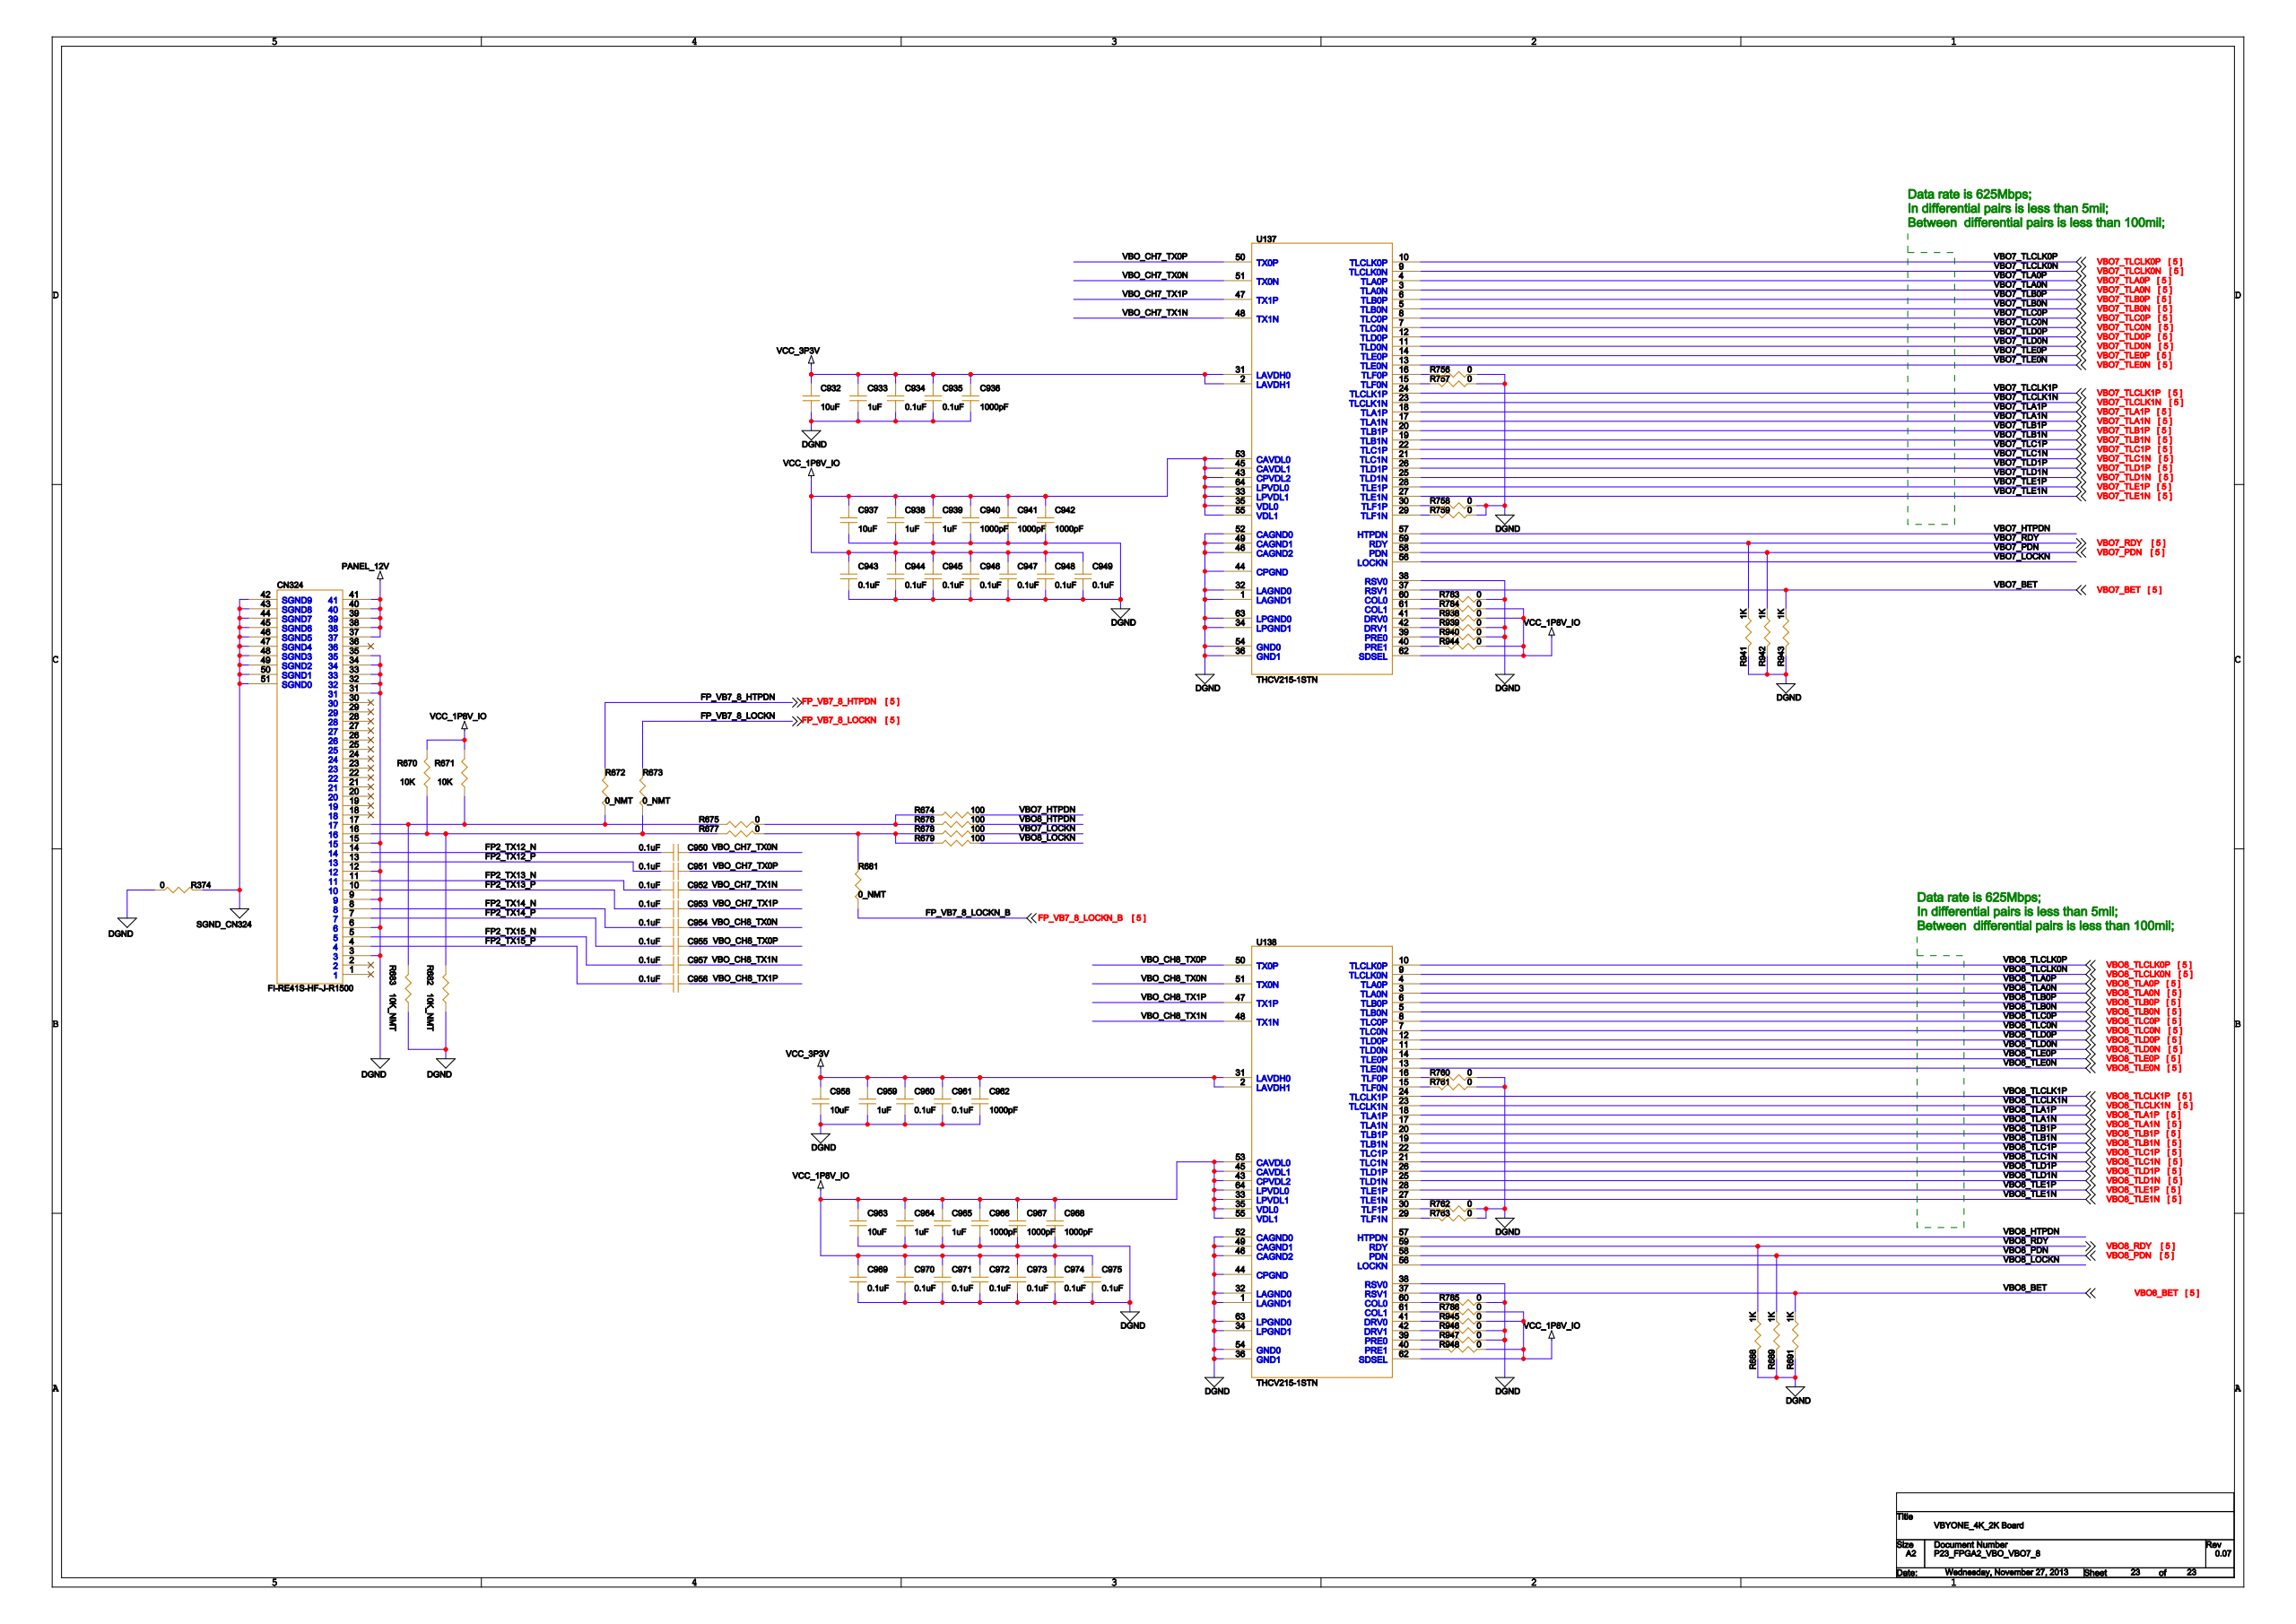Circuit board | Cadence Allegro | 1712 parts | 1495 nets | one sheet of the schematic
Parts on this sheet (reference | value | footprint):
C932 | 10uF | CRC2012RZAS
C933 | 1uF | CRC1608RZAS
C934 | 0.1uF | CRC1005RZAS
C935 | 0.1uF | CRC1005RZAS
C936 | 1000pF | CRC1608RZAS
C937 | 10uF | CRC2012RZAS
C938 | 1uF | CRC1608RZAS
C939 | 1uF | CRC1608RZAS
C940 | 1000pF | CRC1608RZAS
C941 | 1000pF | CRC1608RZAS
C942 | 1000pF | CRC1608RZAS
C943 | 0.1uF | CRC1005RZAS
C944 | 0.1uF | CRC1005RZAS
C945 | 0.1uF | CRC1005RZAS
C946 | 0.1uF | CRC1005RZAS
C947 | 0.1uF | CRC1005RZAS
C948 | 0.1uF | CRC1005RZAS
C949 | 0.1uF | CRC1005RZAS
C950 | 0.1uF | CRC1005RZAS
C951 | 0.1uF | CRC1005RZAS
C952 | 0.1uF | CRC1005RZAS
C953 | 0.1uF | CRC1005RZAS
C954 | 0.1uF | CRC1005RZAS
C955 | 0.1uF | CRC1005RZAS
C956 | 0.1uF | CRC1005RZAS
C957 | 0.1uF | CRC1005RZAS
C958 | 10uF | CRC2012RZAS
C959 | 1uF | CRC1608RZAS
C960 | 0.1uF | CRC1005RZAS
C961 | 0.1uF | CRC1005RZAS
C962 | 1000pF | CRC1608RZAS
C963 | 10uF | CRC2012RZAS
C964 | 1uF | CRC1608RZAS
C965 | 1uF | CRC1608RZAS
C966 | 1000pF | CRC1608RZAS
C967 | 1000pF | CRC1608RZAS
C968 | 1000pF | CRC1608RZAS
C969 | 0.1uF | CRC1005RZAS
C970 | 0.1uF | CRC1005RZAS
C971 | 0.1uF | CRC1005RZAS
C972 | 0.1uF | CRC1005RZAS
C973 | 0.1uF | CRC1005RZAS
C974 | 0.1uF | CRC1005RZAS
C975 | 0.1uF | CRC1005RZAS
CN324 | FI-RE41S-HF-J-R1500 | CAC041RCAS
R374 | 0 | CRC1608RZAS
R670 | 10K | CRC1005RZAS
R671 | 10K | CRC1005RZAS
R672 | 0_NMT | CRC1608RZAS
R673 | 0_NMT | CRC1608RZAS
R674 | 100 | CRC1005RZAS
R675 | 0 | CRC1608RZAS
R676 | 100 | CRC1005RZAS
R677 | 0 | CRC1608RZAS
R678 | 100 | CRC1005RZAS
R679 | 100 | CRC1005RZAS
R681 | 0_NMT | CRC1608RZAS
R682 | 10K_NMT | CRC1005RZAS
R683 | 10K_NMT | CRC1005RZAS
R688 | 1K | CRC1608RZAS
R689 | 1K | CRC1608RZAS
R691 | 1K | CRC1608RZAS
R756 | 0 | CRC1608RZAS
R757 | 0 | CRC1608RZAS
R758 | 0 | CRC1608RZAS
R759 | 0 | CRC1608RZAS
R760 | 0 | CRC1608RZAS
R761 | 0 | CRC1608RZAS
R762 | 0 | CRC1608RZAS
R763 | 0 | CRC1608RZAS
R783 | 0 | CRC1608RZAS
R784 | 0 | CRC1608RZAS
R785 | 0 | CRC1608RZAS
R786 | 0 | CRC1608RZAS
R938 | 0 | CRC1608RZAS
R939 | 0 | CRC1608RZAS
R940 | 0 | CRC1608RZAS
R941 | 1K | CRC1608RZAS
R942 | 1K | CRC1608RZAS
R943 | 1K | CRC1608RZAS
R944 | 0 | CRC1608RZAS
R945 | 0 | CRC1608RZAS
R946 | 0 | CRC1608RZAS
R947 | 0 | CRC1608RZAS
R948 | 0 | CRC1608RZAS
U137 | THCV215-1STN | SOC064RCAT
U138 | THCV215-1STN | SOC064RCAT
Nets of these parts (net: part-pin ...):
VCC_3P3V: C932-2 C933-2 C934-2 C935-2 C936-2 C958-2 C959-2 C960-2 C961-2 C962-2 U137-2 U137-31 U138-2 U138-31
DGND: C932-1 C933-1 C934-1 C935-1 C936-1 C937-1 C938-1 C939-1 C940-1 C941-1 C942-1 C943-1 C944-1 C945-1 C946-1 C947-1 C948-1 C949-1 C958-1 C959-1 C960-1 C961-1 C962-1 C963-1 C964-1 C965-1 C966-1 C967-1 C968-1 C969-1 C970-1 C971-1 C972-1 C973-1 C974-1 C975-1 R374-2 R682-2 R683-2 R688-1 R689-1 R691-1 R756-2 R757-2 R758-2 R759-2 R760-2 R761-2 R762-2 R763-2 R783-2 R785-2 R939-2 R940-2 R941-1 R942-1 R943-1 R946-2 R947-2 CN324-3 CN324-6 CN324-9 CN324-12 CN324-15 CN324-31 CN324-32 CN324-33 CN324-34 CN324-35 U137-1 U137-32 U137-34 U137-36 U137-38 U137-44 U137-46 U137-49 U137-52 U137-54 U137-63 U138-1 U138-32 U138-34 U138-36 U138-38 U138-44 U138-46 U138-49 U138-52 U138-54 U138-63
VCC_1P8V_IO: C937-2 C938-2 C939-2 C940-2 C941-2 C942-2 C943-2 C944-2 C945-2 C946-2 C947-2 C948-2 C949-2 C963-2 C964-2 C965-2 C966-2 C967-2 C968-2 C969-2 C970-2 C971-2 C972-2 C973-2 C974-2 C975-2 R670-1 R671-1 R784-2 R786-2 R938-2 R944-2 R945-2 R948-2 U137-33 U137-35 U137-43 U137-45 U137-53 U137-55 U137-62 U137-64 U138-33 U138-35 U138-43 U138-45 U138-53 U138-55 U138-62 U138-64
PANEL_12V: CN324-37 CN324-38 CN324-39 CN324-40 CN324-41
VBO_CH7_TX0N: C950-1 U137-51
FP2_TX12_N: C950-2 CN324-14
VBO_CH7_TX0P: C951-1 U137-50
FP2_TX12_P: C951-2 CN324-13
VBO_CH7_TX1N: C952-1 U137-48
FP2_TX13_N: C952-2 CN324-11
VBO_CH7_TX1P: C953-1 U137-47
FP2_TX13_P: C953-2 CN324-10
VBO_CH8_TX0N: C954-1 U138-51
FP2_TX14_N: C954-2 CN324-8
VBO_CH8_TX0P: C955-1 U138-50
FP2_TX14_P: C955-2 CN324-7
VBO_CH8_TX1P: C956-1 U138-47
FP2_TX15_P: C956-2 CN324-4
VBO_CH8_TX1N: C957-1 U138-48
FP2_TX15_N: C957-2 CN324-5
SGND_CN324: R374-1 CN324-42 CN324-43 CN324-44 CN324-45 CN324-46 CN324-47 CN324-48 CN324-49 CN324-50 CN324-51
N19776221: R670-2 R673-2 R677-2 R682-1 CN324-16
N19776219: R671-2 R672-2 R675-2 R683-1 CN324-17
N19777273: R674-2 R675-1 R676-2
N19777369: R677-1 R678-2 R679-2 R681-1
FP_VB7_8_HTPDN: R672-1
FP_VB7_8_LOCKN: R673-1
FP_VB7_8_LOCKN_B: R681-2
VBO7_HTPDN: R674-1 U137-57
VBO8_HTPDN: R676-1 U138-57
VBO7_LOCKN: R678-1 U137-56
VBO8_LOCKN: R679-1 U138-56
VBO8_RDY: R688-2 U138-59
VBO8_PDN: R689-2 U138-58
VBO8_BET: R691-2 U138-37
VBO7_RDY: R941-2 U137-59
VBO7_PDN: R942-2 U137-58
VBO7_BET: R943-2 U137-37
N19924396: R756-1 U137-16
N19924386: R757-1 U137-15
N19926463: R758-1 U137-30
N19926660: R759-1 U137-29
N19924697: R760-1 U138-16
N19924687: R761-1 U138-15
N19924906: R762-1 U138-30
N19924907: R763-1 U138-29
N20037576: R783-1 U137-60
N20037771: R784-1 U137-61
N20038211: R785-1 U138-60
N20038406: R786-1 U138-61
N19776279: R938-1 U137-41
N19776277: R939-1 U137-42
N19776285: R940-1 U137-39
N19776289: R944-1 U137-40
N19921780: R945-1 U138-41
N19921784: R946-1 U138-42
N19921794: R947-1 U138-39
N19921799: R948-1 U138-40
VBO7_TLE1P: U137-28
VBO7_TLE1N: U137-27
VBO7_TLCLK1P: U137-24
VBO7_TLC1P: U137-22
VBO8_TLE1P: U138-28
VBO8_TLE1N: U138-27
VBO8_TLCLK1P: U138-24
VBO8_TLCLK1N: U138-23
VBO8_TLA0P: U138-4
VBO7_TLA1P: U137-18
VBO7_TLCLK1N: U137-23
VBO7_TLC1N: U137-21
VBO8_TLB0P: U138-6
VBO8_TLD1P: U138-26
VBO8_TLB1P: U138-20
VBO8_TLB1N: U138-19
VBO8_TLA0N: U138-3
VBO7_TLA1N: U137-17
VBO7_TLD0P: U137-12
VBO7_TLD0N: U137-11
VBO7_TLD1P: U137-26
VBO7_TLD1N: U137-25
VBO8_TLB0N: U138-5
VBO8_TLD1N: U138-25
VBO8_TLC0P: U138-8
VBO8_TLC0N: U138-7
VBO7_TLB1P: U137-20
VBO7_TLB1N: U137-19
VBO7_TLE0P: U137-14
VBO7_TLE0N: U137-13
VBO8_TLA1P: U138-18
VBO8_TLC1P: U138-22
VBO8_TLC1N: U138-21
VBO8_TLD0P: U138-12
VBO7_TLC0P: U137-8
VBO7_TLC0N: U137-7
VBO7_TLCLK0P: U137-10
VBO7_TLCLK0N: U137-9
VBO8_TLE0P: U138-14
VBO8_TLA1N: U138-17
VBO8_TLCLK0P: U138-10
VBO8_TLCLK0N: U138-9
VBO8_TLD0N: U138-11
VBO7_TLA0P: U137-4
VBO7_TLA0N: U137-3
VBO7_TLB0P: U137-6
VBO7_TLB0N: U137-5
VBO8_TLE0N: U138-13